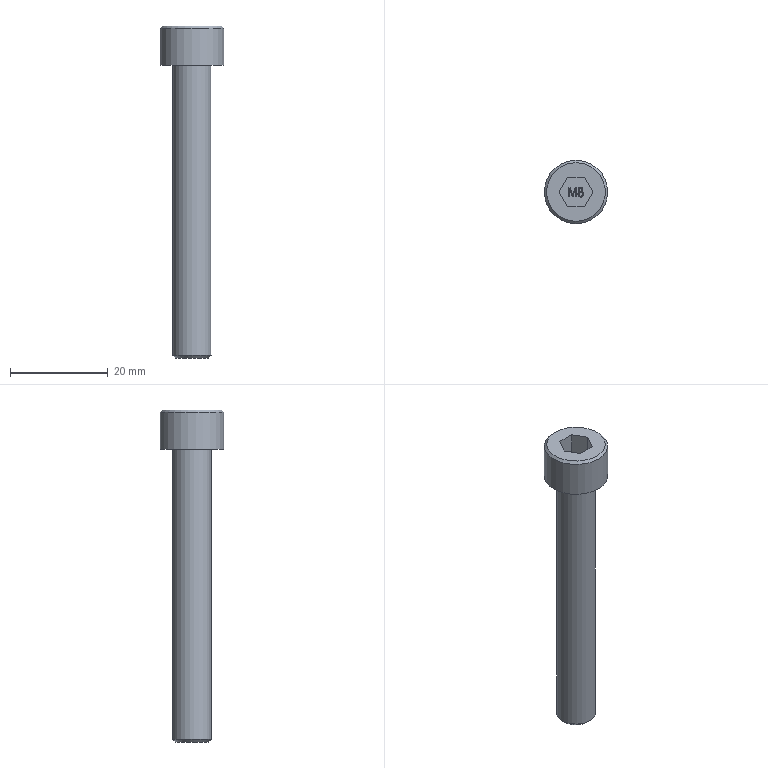Part | STEP file | SOLID | 1 solid | 38 faces | box 13 x 13 x 68 mm | volume 3913 mm3 | plane 25 | other 9 | cylinder 2 | cone 2 | commonest cylinder face diameters 8 x1 13 x1